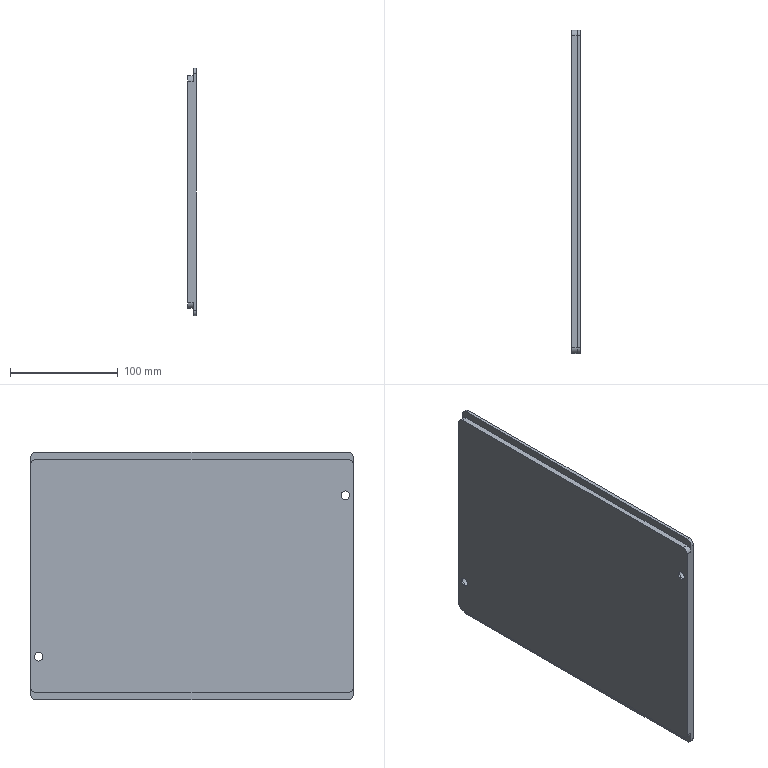Part | STEP file | 1 solid | 36 faces | box 8 x 300 x 230 mm | volume 529041 mm3 | plane 20 | cylinder 16 | commonest cylinder face diameters 10 x8 8 x4 12 x4